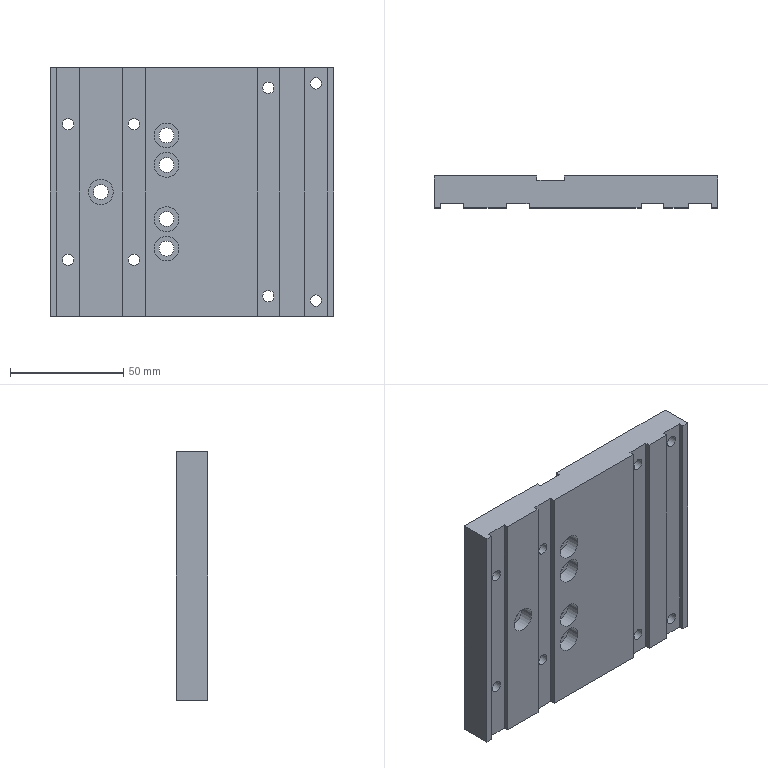CAM job | NX | 3-axis milling, drilling | part box 125.5 x 14 x 110 mm | stock box 135.5 x 24 x 110 mm
Tools:
number,name,description,diameter,corner_radius,flute_length,length,flutes
0,D8,Milling Tool-5 Parameters,8.0,0.0,50.0,75.0,2
0,D12,Milling Tool-5 Parameters,12.0,0.0,50.0,75.0,2
0,D6,Milling Tool-5 Parameters,6.0,0.0,50.0,75.0,2
Operations:
program,operation,operation_type,tool,method,geometry_group,spindle_rpm,surface_speed,feed_per_tooth,feed_cut,feed_plunge,cut_length_mm,path_length_mm,cut_time_min,machine_time_min
NC_PROGRAM,PLANAR_PROFILE,PlanarMilling,D12,METHOD,WORKPIECE,0.0,0.0,0.0,250.0,100.0,14980.0,15048.0,59.92,59.927
NC_PROGRAM,FLOOR_WALL,VolumeBased25DMillingOperation,D8,METHOD,WORKPIECE,0.0,0.0,0.0,250.0,100.0,5006.0,5275.743,20.024,20.051
NC_PROGRAM,FLOOR_WALL_COPY,VolumeBased25DMillingOperation,D8,METHOD,WORKPIECE,0.0,0.0,0.0,250.0,100.0,1000.0,1248.5,4.0,4.025
NC_PROGRAM,SPOT_DRILLING,Operation,D8,METHOD,WORKPIECE,0.0,0.0,0.0,250.0,0.0,39.0,595.97,0.156,0.2117
NC_PROGRAM,HOLE_MILLING,CylinderMilling,D6,METHOD,WORKPIECE,0.0,0.0,0.0,250.0,100.0,556.458,908.217,2.226,2.261